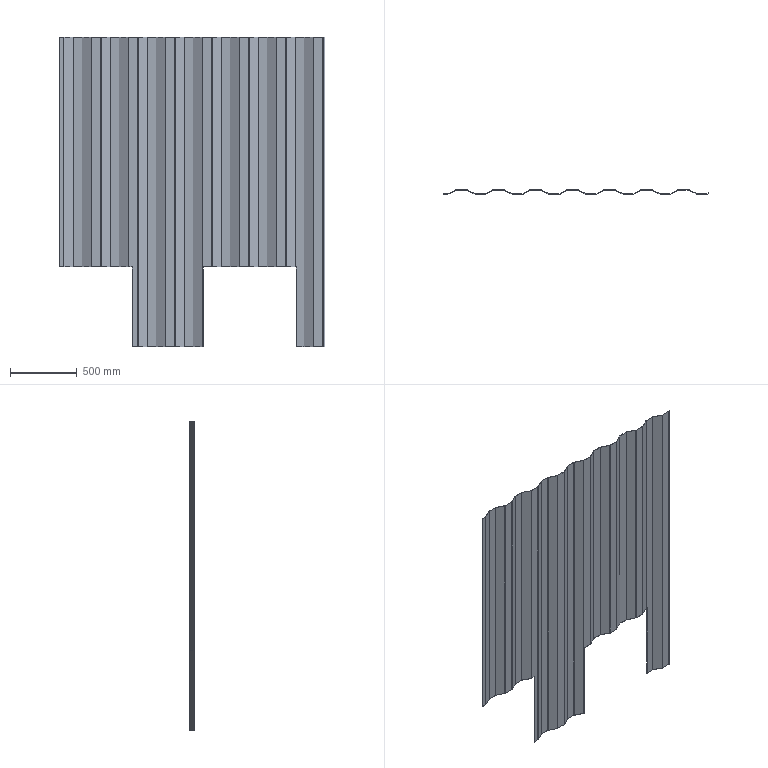Part | STEP file | 750038178 | 1 solid | 128 faces | box 1997 x 36 x 2327 mm | volume 8230400 mm3 | plane 70 | cylinder 58 | commonest cylinder face diameters 6 x29 10 x29